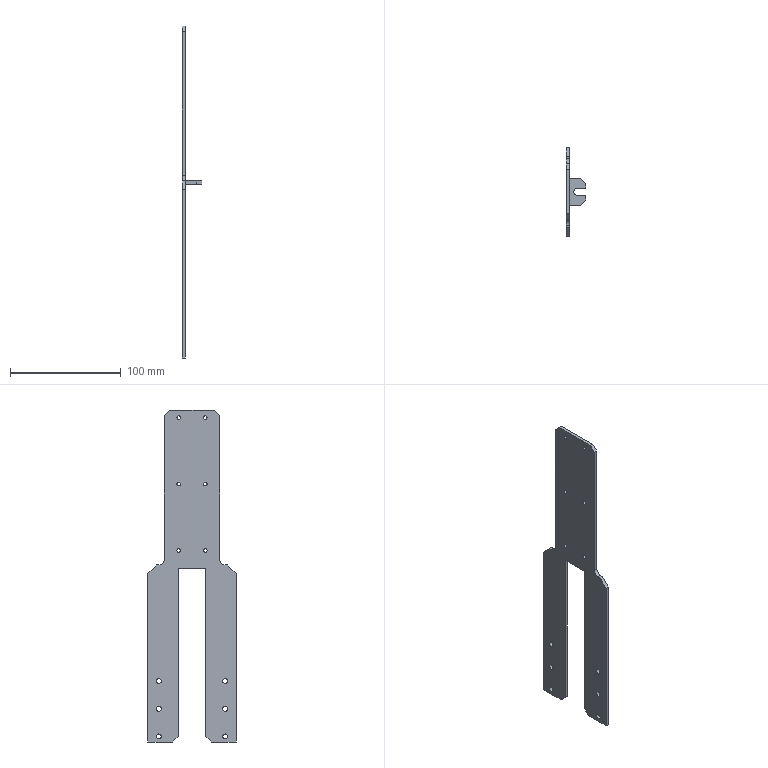Part | SolidWorks | features ICE 7, Chamfer 4, LPattern 2, 3DProfileFeature 1, Extrusion 1, Fillet 1, HoleWzd 1 | 1 solid | 57 faces | box 18 x 80 x 300 mm | volume 47731 mm3 | plane 29 | cylinder 28 | commonest cylinder face diameters 3.3 x12 4.5 x12 6.2 x2 10 x2